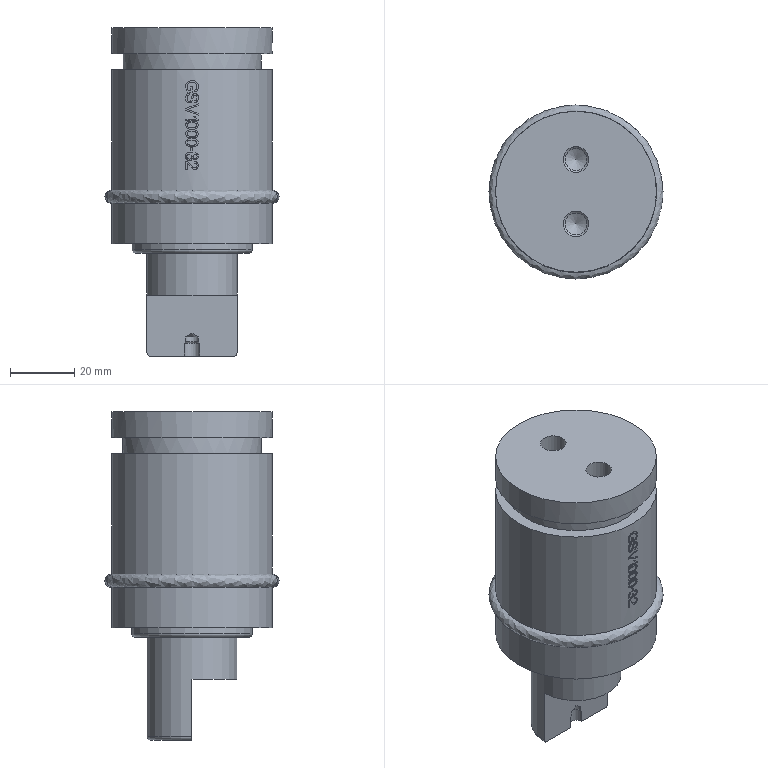Part | NX | features solid 2 | 1 solid | 187 faces | box 54.1 x 54.1 x 102 mm | volume 146219 mm3 | plane 94 | cylinder 84 | cone 6 | torus 2 | spline 1 | commonest cylinder face diameters 49.8 x10 50 x6 1.621 x3 1.934 x3 1.94 x3 1.962 x3